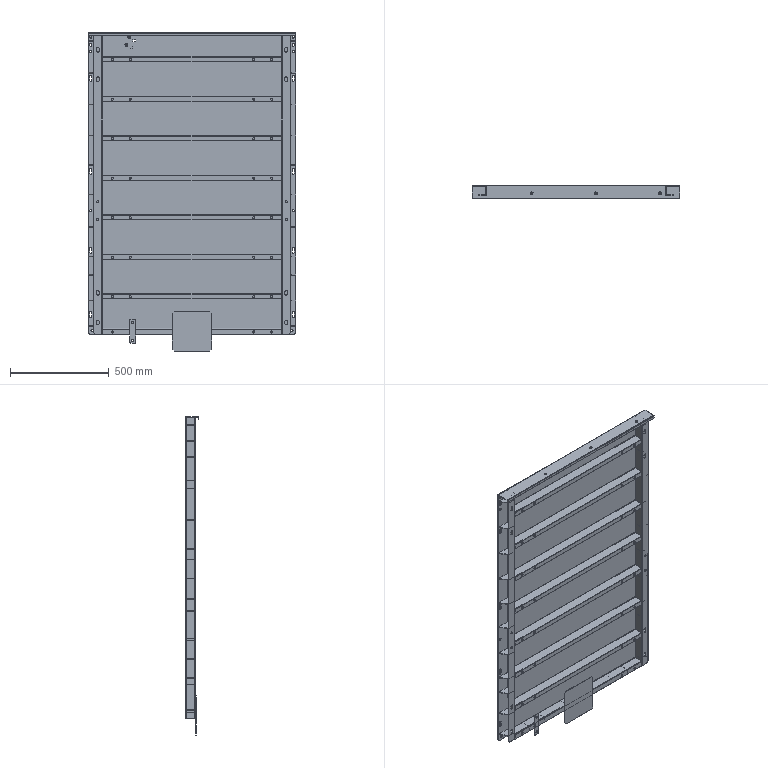Part | SolidWorks | features ReferencePattern 32, LocalLPattern 5, MirrorCompFeat 5 | 48 solids | 1020 faces | box 1050 x 70 x 1610 mm | volume 8250667 mm3 | plane 636 | cylinder 354 | cone 30 | commonest cylinder face diameters 11 x140 10 x88 12 x24 0.4 x22 4.4 x14 6.917 x10